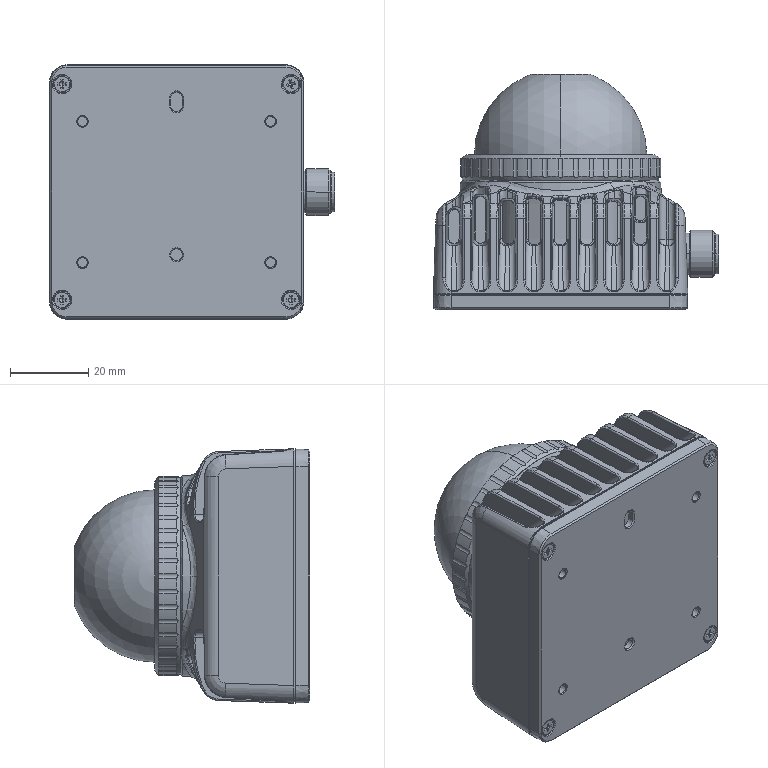Part | SolidWorks | 7 solids | 1763 faces | box 72.737 x 60.097 x 64.874 mm | volume 142272 mm3 | cylinder 591 | plane 461 | spline 342 | cone 226 | torus 137 | sphere 6 | commonest cylinder face diameters 0.8 x102 3.2 x87 0.6 x74 2 x64 51 x40 0.3 x32